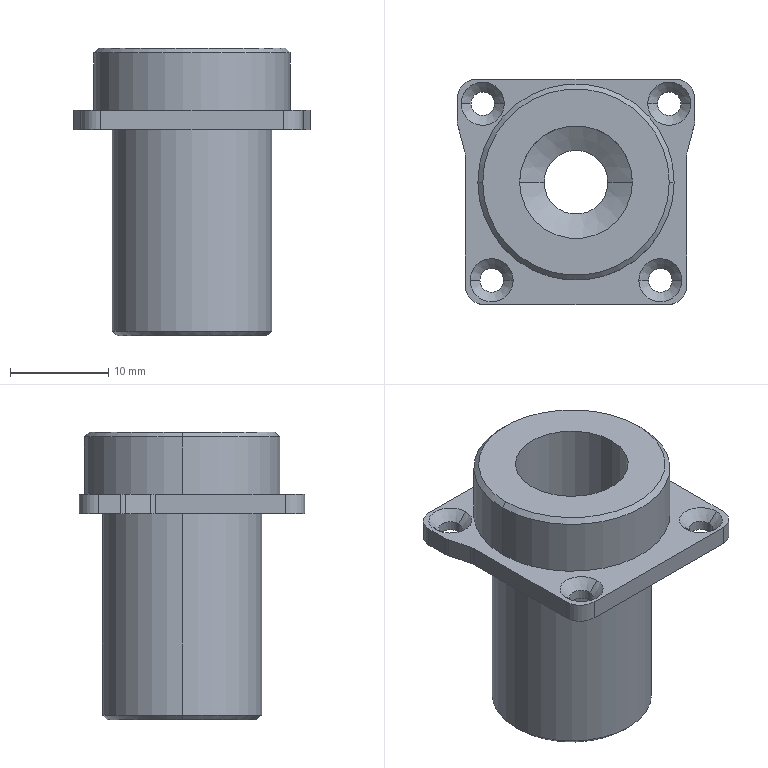NC program | NX | posted with a generic post | part box 24.2 x 23 x 29.342 mm
Lines 1 to 754 of 2259:
N10 G17 G21 G94 G90
(动态粗_2 , TOOL : D8-25-D8-60-3T-ROUGH)
N12 T02 M6
N14 G54
N16 G17 G0 G90 X-22.512 Y5.441 S6500 M3
N18 G43 Z20. H2
N20 Z-7.845
N22 G94 G1 X-22.487 Y5.442 Z-8.001 F3000.
N24 X-22.462 Y5.443 Z-8.063
N26 X-22.437 Y5.444 Z-8.109
N28 X-22.412 Y5.445 Z-8.145
N30 X-22.387 Y5.446 Z-8.176
N32 X-22.362 Y5.447 Z-8.202
N34 X-22.337 Y5.448 Z-8.225
N36 X-22.312 Y5.45 Z-8.245
N38 X-22.287 Y5.451 Z-8.263
N40 X-22.262 Y5.452 Z-8.278
N42 X-22.237 Y5.453 Z-8.292
N44 X-22.212 Y5.454 Z-8.303
N46 X-22.187 Y5.455 Z-8.314
N48 X-22.162 Y5.456 Z-8.322
N50 X-22.137 Y5.457 Z-8.329
N52 X-22.112 Y5.459 Z-8.335
N54 X-22.087 Y5.46 Z-8.34
N56 X-22.062 Y5.461 Z-8.343
N58 X-22.037 Y5.462 Z-8.345
N60 X-22.012 Y5.463
N62 X-20.703 Y5.522
N64 G3 X-20. Y6.002 R0.809
N66 X-19.572 Y8.199 R7.463
N68 X-19.395 Y13.319 R106.579
N70 G2 X-17.366 Y16.534 R4.682
N72 X-13.438 Y18.014 R9.169
N74 X-8.009 Y18.368 R38.584
N76 G1 X0.271 Y18.398
N78 X14.049 Y18.397
N80 G2 X17.314 Y16.635 R4.483
N82 X18.942 Y12.823 R8.468
N84 X19.358 Y7.581 R32.221
N86 X19.398 Y-1.284 R659.911
N88 G1 X19.397 Y-15.017
N90 G2 X17.621 Y-18.322 R4.482
N92 X13.889 Y-19.928 R8.428
N94 X8.423 Y-20.361 R32.437
N96 X-0.352 Y-20.398 R663.379
N98 G1 X-14.049 Y-20.397
N100 G2 X-17.315 Y-18.63 R4.484
N102 X-18.954 Y-14.756 R8.529
N104 X-19.359 Y-9.512 R32.975
N106 X-19.379 Y3.952 R670.697
N108 G3 X-18.957 Y8.894 R317.041
N110 G2 X-18.812 Y11.634 R51.298
N112 X-15.837 Y15.936 R6.134
N114 X-11.501 Y17.394 R11.47
N116 X-5.037 Y17.773 R48.523
N118 G1 X2.882 Y17.798
N120 X12.266 Y17.782
N122 G2 X16.841 Y14.939 R5.988
N124 X18.373 Y10.596 R11.098
N126 X18.767 Y4.449 R44.394
N128 G1 X18.798 Y-3.966
N130 X18.782 Y-13.258
N132 G2 X16.002 Y-17.798 R5.972
N134 X11.573 Y-19.376 R11.04
N136 X5.426 Y-19.767 R44.614
N138 G1 X-2.989 Y-19.798
N140 X-12.258 Y-19.783
N142 G2 X-16.766 Y-17.05 R5.959
N144 X-18.36 Y-12.674 R10.881
N146 X-18.766 Y-6.483 R43.41
N148 X-18.765 Y3.057 R288.24
N150 X-18.286 Y10.04 R540.807
N152 X-14.554 Y15.361 R7.081
N154 X-9.803 Y16.81 R13.416
N156 X-2.752 Y17.176 R58.621
N158 X10.578 Y17.182 R835.39
N160 X16.232 Y13.697 R6.869
N162 X17.769 Y9.019 R12.685
N164 X18.164 Y2.646 R49.478
N166 X18.179 Y-11.629 R815.472
N168 X14.718 Y-17.217 R6.865
N170 X9.955 Y-18.778 R12.739
N172 X3.312 Y-19.169 R51.931
N174 X-10.683 Y-19.176 R655.475
N176 X-16.201 Y-15.746 R6.857
N178 X-17.754 Y-11.114 R12.528
N180 X-18.162 Y-4.787 R47.586
N182 X-18.083 Y3.94 R125.28
N184 X-17.739 Y8.81 R94.032
N186 X-13.528 Y14.722 R7.786
N188 X-8.497 Y16.2 R14.685
N190 X-1.265 Y16.573 R62.487
N192 X9.296 Y16.571 R383.455
N194 X15.664 Y12.521 R7.559
N196 X17.18 Y7.555 R14.271
N198 X17.566 Y0.776 R56.697
N200 X17.571 Y-10.288 R389.819
N202 X13.525 Y-16.66 R7.554
N204 X8.517 Y-18.185 R14.229
N206 X1.647 Y-18.568 R57.833
N208 X-9.288 Y-18.571 R390.256
N210 X-15.634 Y-14.572 R7.543
N212 X-17.153 Y-9.744 R13.906
N214 X-17.567 Y-2.696 R55.095
N216 X-17.217 Y7.463 R91.433
N218 X-14.761 Y12.546 R8.264
N220 G1 X-14.483 Y12.885
N222 G2 X-13.313 Y13.797 R9.766
N224 X-7.944 Y15.517 R15.205
N226 X-0.852 Y15.958 R55.535
N228 X7.967 Y15.969 R285.236
N230 X13.459 Y13.7 R8.163
N232 X14.491 Y12.877 R12.481
N234 G1 X15.259 Y11.938
N236 X15.83 Y10.867
N238 G2 X16.465 Y7.974 R13.069
N240 X16.957 Y0.03 R64.584
N242 X16.966 Y-9.015 R263.202
N244 X12.547 Y-16.03 R8.091
N246 X7.395 Y-17.566 R15.148
N248 X0.12 Y-17.966 R60.98
N250 X-8.114 Y-17.961 R206.184
N252 X-15.037 Y-13.536 R8.082
N254 X-16.55 Y-8.516 R15.03
N256 X-16.96 Y-0.973 R58.274
N258 X-16.652 Y6.443 R70.854
N260 X-16.3 Y8.206 R24.664
N262 X-16.18 Y9.711 R13.074
N264 G1 X-15.827 Y10.874
N266 X-15.254 Y11.946
N268 X-14.483 Y12.885
N270 X-13.543 Y13.656
N272 X-12.471 Y14.228
N274 X-11.308 Y14.581
N276 G2 X-4.847 Y15.189 R185.641
N278 X7.07 Y15.342 R157.749
N280 X10.118 Y14.7 R10.992
N282 G1 X11.326 Y14.577
N284 X12.486 Y14.222
N286 X13.477 Y13.69
N288 X12.486 Y14.222
N290 X11.326 Y14.577
N292 G3 X6.199 Y14.972 R82.367
N294 X-7.446 Y15.01 R819.421
N296 G2 X-8.114 Y15.371 R0.802
N298 G1 X-9.01 Y16.671 Z-8.245
N300 X-9.193 Y16.933 F15000.
N302 X-9.363 Y17.204
N304 G2 X-9.18 Y18.131 R0.807
N306 X-8.379 Y16.814 R-0.8
N308 G1 X-8.857 Y16.68
N310 X-10.376 Y16.251 Z-8.345 F3000.
N312 G3 X-10.099 Y14.7 R0.8
N314 G1 X10.061
N316 X11.326 Y14.577
N318 X12.486 Y14.222
N320 X13.555 Y13.648
N322 X14.491 Y12.877
N324 X15.259 Y11.938
N326 X15.83 Y10.867
N328 X16.181 Y9.706
N330 X16.3 Y8.499
N332 G3 X16.367 Y-1.226 R300.802
N334 G2 X16.368 Y-7.896 R177.779
N336 X15.332 Y-11.87 R9.377
N338 G1 X15.027 Y-12.874
N340 X14.454 Y-13.946
N342 X13.683 Y-14.885
N344 X12.743 Y-15.656
N346 X11.671 Y-16.228
N348 X10.508 Y-16.581
N350 G3 X6.375 Y-17.049 R499.901
N352 G2 X-3.864 Y-17.379 R115.219
N354 X-7.735 Y-17.282 R36.54
N356 X-10.338 Y-16.601 R10.078
N358 X-11.674 Y-16.227 R8.73
N360 G1 X-12.746 Y-15.654
N362 X-13.685 Y-14.883
N364 X-14.456 Y-13.943
N366 X-15.028 Y-12.871
N368 G2 X-15.673 Y-10.053 R14.491
N370 X-16.333 Y-0.447 R58.318
N372 X-16.152 Y4.948 R96.408
N374 X-16.3 Y6.249 R6.163
N376 G1 Y8.229
N378 G3 X-16.247 Y5.441 R30.966
N380 G2 X-15.973 Y2.291 R13.081
N382 G3 X-15.702 Y-6.763 R98.047
N384 G1 X-15.504 Y-8.552
N386 X-15.5 Y-10.499
N388 X-15.381 Y-11.708
N390 X-15.5 Y-10.499
N392 X-15.534 Y2.547
N394 X-16.098 Y4.689
N396 G3 X-17.144 Y5.289 R0.8
N398 X-17.654 Y4.757 Z-8.297 R0.837
N400 G1 X-17.952 Y3.999 Z-8.245
N402 X-18.275 Y3.189 F15000.
N404 X-18.585 Y2.375
N406 X-18.609 Y2.177
N408 Y-3.989
N410 G3 X-17.885 Y-11.32 R37.463
N412 G1 X-17.731 Y-12.099
N414 X-17.563 Y-12.875
N416 G3 X-15.309 Y-16.66 R7.761
N418 G1 X-13.459 Y-18.369
N420 G3 X-12.311 Y-18.305 R0.8
N422 G1 X-12.182 Y-18.156
N424 X-11.149 Y-16.962 Z-8.345 F3000.
N426 G2 X-10.51 Y-16.591 R0.883
N428 G1 X-7.5 Y-16.9
N430 G3 X5.99 Y-16.7 R112.077
N432 G1 X9.299
N434 X-9.301
N436 X-9.928 Y-16.638
N438 G3 X-10.397 Y-18.132 R0.8
N440 G1 X-10.016 Y-18.283 Z-8.319
N442 X-9.629 Y-18.416 Z-8.293
N444 X-8.913 Y-18.669 Z-8.245
N446 X-7.683 Y-19.104 F15000.
N448 X-7.551 Y-19.137
N450 X-7.416 Y-19.15
N452 X8.372
N454 G3 X12.628 Y-18.396 R12.335
N456 X15.501 Y-16.541 R8.304
N458 G1 X17.108 Y-14.947
N460 G3 X17.007 Y-13.725 R0.8
N462 G1 X16.874 Y-13.632
N464 X15.587 Y-12.718 Z-8.345 F3000.
N466 G2 X15.332 Y-11.87 R0.801
N468 G3 X15.999 Y-5.757 R26.509
N470 X15.938 Y4.056 R319.266
N472 X16.285 Y6.022 R7.695
N474 G2 X15.948 Y4.118 R7.088
N476 G3 X15.5 Y0.932 R11.588
N478 G1 Y-10.501
N480 X15.38 Y-11.711
N482 X15.5 Y-10.501
N484 G2 X15.516 Y2.489 R970.595
N486 G1 X15.745 Y3.362
N488 G2 X16.658 Y3.95 R0.808
N490 G1 X17.894 Y3.745
N492 X17.919 Y3.741
N494 X17.943 Y3.737 Z-8.343
N496 X17.968 Y3.733 Z-8.34
N498 X17.993 Y3.729 Z-8.335
N500 X18.017 Y3.725 Z-8.329
N502 X18.042 Y3.721 Z-8.322
N504 X18.067 Y3.717 Z-8.314
N506 X18.091 Y3.713 Z-8.303
N508 X18.116 Y3.708 Z-8.292
N510 X18.141 Y3.704 Z-8.278
N512 X18.165 Y3.7 Z-8.263
N514 X18.19 Y3.696 Z-8.245
N516 X18.215 Y3.692 Z-8.225
N518 X18.239 Y3.688 Z-8.202
N520 X18.264 Y3.684 Z-8.176
N522 X18.289 Y3.68 Z-8.145
N524 X18.313 Y3.676 Z-8.109
N526 X18.338 Y3.672 Z-8.063
N528 X18.363 Y3.668 Z-8.001
N530 X18.387 Y3.664 Z-7.845
N532 G0 Z20.
N534 X-18.056 Y-0.544
N536 Z-5.692
N538 G1 X-18.031 Y-0.543 Z-5.848
N540 X-18.006 Y-0.541 Z-5.91
N542 X-17.981 Y-0.54 Z-5.955
N544 X-17.956 Y-0.539 Z-5.992
N546 X-17.931 Y-0.538 Z-6.023
N548 X-17.906 Y-0.537 Z-6.049
N550 X-17.881 Y-0.535 Z-6.072
N552 X-17.856 Y-0.534 Z-6.092
N554 X-17.831 Y-0.533 Z-6.11
N556 X-17.806 Y-0.532 Z-6.125
N558 X-17.781 Y-0.53 Z-6.139
N560 X-17.757 Y-0.529 Z-6.15
N562 X-17.732 Y-0.528 Z-6.16
N564 X-17.707 Y-0.527 Z-6.169
N566 X-17.682 Y-0.526 Z-6.176
N568 X-17.657 Y-0.524 Z-6.182
N570 X-17.632 Y-0.523 Z-6.186
N572 X-17.607 Y-0.522 Z-6.189
N574 X-17.582 Y-0.521 Z-6.191
N576 X-17.557 Y-0.52 Z-6.192
N578 X-16.242 Y-0.456
N580 G3 X-15.544 Y0.02 R0.809
N582 X-15.265 Y2.979 R5.282
N584 G2 X-15.573 Y7.824 R21.945
N586 X-11.556 Y13.104 R6.034
N588 X-7.333 Y13.936 R14.619
N590 X-1.626 Y14.093 R100.555
N592 X1.604 Y14.151 R18.527
N594 G1 X8.859 Y14.082
N596 G2 X13.059 Y12.48 R6.527
N598 X15.067 Y8.869 R7.229
N600 X15.196 Y4.756 R10.856
N602 G3 X14.924 Y-0.404 R42.779
N604 G2 X14.876 Y-9.366 R674.909
N606 X13.175 Y-13.57 R6.436
N608 X9.53 Y-15.501 R7.476
N610 X4.482 Y-16.039 R24.687
N612 X-8.127 Y-16.077 R423.69
N614 X-12.348 Y-14.396 R6.459
N616 X-14.299 Y-10.757 R7.365
N618 X-14.836 Y-5.8 R24.291
N620 X-14.827 Y-1.258 R45.147
N622 G3 X-14.744 Y2.734 R19.949
N624 G2 X-14.905 Y6.411 R31.666
N626 X-11.612 Y11.716 R6.376
N628 X-7.086 Y13.138 R12.123
N630 G1 X-4.76 Y13.378
N632 X-3.102 Y13.857
N634 X-1.383 Y14.132
N636 X0.403 Y14.192
N638 X2.093 Y14.045
N640 G3 X6.185 Y13.573 R18.076
N642 G2 X9.306 Y13.257 R14.034
N644 X13.888 Y8.721 R6.619
N646 X14.379 Y4.942 R12.987
N648 G1 X14.313 Y-2.676
N650 G2 X14.26 Y-8.243 R144.693
N652 X10.572 Y-13.892 R6.619
N654 X5.915 Y-15.194 R13.228
N656 X-1.185 Y-15.485 R68.155
N658 X-7.079 Y-15.455 R116.893
N660 X-12.675 Y-11.812 R6.599
N662 X-13.985 Y-7.205 R13.045
N664 X-14.149 Y-0.973 R35.635
N666 X-14.163 Y1.031 R16.707
N668 X-14.256 Y4.941 R219.386
N670 X-10.671 Y10.939 R7.006
N672 X-7.102 Y12.277 R12.297
N674 G1 X-6.377 Y12.687
N676 X-4.732 Y13.385
N678 X-6.377 Y12.687
N680 G2 X-8.857 Y11.422 R20.302
N682 G3 X-12.298 Y8.661 R8.483
N684 X-13.649 Y4.605 R8.528
N686 G2 X-13.773 Y3.456 R6.931
N688 G1 X-14.092 Y1.744
N690 X-14.167 Y0.531
N692 X-14.092 Y1.744
N694 X-13.742 Y3.554
N696 G2 X-12.416 Y6.912 R16.172
N698 X-10.517 Y9.542 R17.949
N700 G1 X-9.269 Y10.757
N702 X-7.882 Y11.811
N704 X-7.221 Y12.196
N706 X-7.882 Y11.811
N708 X-9.269 Y10.757
N710 X-10.517 Y9.542
N712 X-11.606 Y8.182
N714 X-12.52 Y6.7
N716 X-13.246 Y5.116
N718 X-13.773 Y3.456
N720 X-14.092 Y1.744
N722 X-14.2 Y0.004
N724 G3 X-13.974 Y-2.692 R28.349
N726 X-13.515 Y-7.605 R57.009
N728 X-12.028 Y-11.772 R10.612
N730 X-7.667 Y-14.66 R6.957
N732 X-3.062 Y-15.096 R22.248
N734 X5.121 Y-14.877 R76.871
N736 X9.681 Y-13.731 R13.656
N738 X13.423 Y-9.021 R6.858
N740 X13.904 Y-4.555 R20.928
N742 G1 X13.948 Y-2.531
N744 X14.103 Y-1.654
N746 X14.2 Y0.004
N748 G2 X13.998 Y5.092 R101.103
N750 G3 X13.131 Y9.065 R10.136
N752 X8.801 Y12.596 R6.693
N754 X5.116 Y13.223 R23.127
N756 X3.14 Y13.819 R10.596
N758 G2 X5.078 Y13.234 R10.018
N760 G3 X8.199 Y12.127 R272.114
N762 G2 X12.61 Y7.306 R7.44
N764 X13.059 Y5.548 R30.574
N766 X13.727 Y3.635 R21.709
N768 X14.093 Y1.655 R23.357
N770 G3 X13.727 Y3.635 R23.357
N772 X13.059 Y5.548 R21.709
N774 X11.888 Y8.013 R55.543
N776 X8.824 Y11.12 R8.285
N778 G1 X7.251 Y12.209
N780 X5.616 Y13.042
N782 X7.251 Y12.209
N784 X8.824 Y11.12
N786 X10.133 Y9.948
N788 X11.331 Y8.558
N790 X12.34 Y7.025
N792 X13.143 Y5.375
N794 X13.727 Y3.635
N796 X14.081 Y1.835
N798 X14.2 Y0.004
N800 G2 X13.814 Y-3.29 R16.567
N802 G3 X13.323 Y-5.938 R16.464
N804 G2 X12.42 Y-9.408 R11.858
N806 X8.318 Y-13.166 R7.767
N808 X3.42 Y-14.277 R16.444
N810 X-5.209 Y-14.332 R51.279
N812 X-9.147 Y-13.043 R8.477
N814 X-12.198 Y-8.926 R8.259
N816 X-12.984 Y-5.74 R18.647
N818 X-14.055 Y-1.907 R14.192
N820 G3 X-12.804 Y-6.147 R14.594
N822 X-11.609 Y-9.212 R35.123
N824 X-6.191 Y-13.549 R7.933
N826 X-1.88 Y-14.058 R19.593
N828 G1 X-0.404 Y-14.194
N830 G3 X6.165 Y-13.399 R29.845
N832 X10.388 Y-11.103 R9.034
N834 X12.558 Y-7.054 R9.04
N836 G1 X12.801 Y-6.112
N838 G3 X13.711 Y-3.63 R13.2
N840 G2 X12.801 Y-6.112 R13.081
N842 X11.84 Y-7.839 R16.008
N844 X8.28 Y-11.519 R9.586
N846 G1 X8.083 Y-11.675
N848 X6.542 Y-12.603
N850 X4.895 Y-13.329
N852 X3.17 Y-13.841
N854 X1.395 Y-14.131
N856 X3.17 Y-13.841
N858 X4.895 Y-13.329
N860 X6.542 Y-12.603
N862 X8.083 Y-11.675
N864 X9.494 Y-10.559
N866 X10.753 Y-9.274
N868 X11.84 Y-7.839
N870 G2 X13.069 Y-7.784 R0.8
N872 X13.268 Y-8.467 Z-6.145 R0.84
N874 G1 X13.196 Y-9.307 Z-6.092
N876 X13.076 Y-10.699 F15000.
N878 G2 X12.759 Y-11.271 R0.803
N880 G1 X11.494 Y-12.224
N882 X10.218 Y-13.163
N884 G2 X6.565 Y-15.249 R22.592
N886 X4.719 Y-15.989 R14.369
N888 X2.475 Y-16.419 R10.72
N890 G1 X0.632 Y-16.57
N892 G2 X-0.125 Y-16.177 R0.805
N894 G1 X-0.993 Y-14.858 Z-6.192 F3000.
N896 X-1.169 Y-14.585
N898 X-1.358 Y-14.32
N900 G3 X-1.88 Y-14.058 R0.805
N902 G1 X-2.195 Y-14.029
N904 G2 X-6.949 Y-12.534 R20.191
N906 X-9.68 Y-10.357 R8.581
N908 G1 X-10.079 Y-10.003
N910 X-11.263 Y-8.648
N912 X-12.266 Y-7.154
N914 X-12.925 Y-5.874
N916 X-12.266 Y-7.154
N918 X-11.263 Y-8.648
N920 X-10.079 Y-10.003
N922 X-8.733 Y-11.197
N924 X-7.247 Y-12.211
N926 X-5.645 Y-13.03
N928 X-4.205 Y-13.548
N930 G2 X-3.673 Y-14.371 R0.808
N932 G1 X-3.777 Y-15.699
N934 X-3.779 Y-15.724 Z-6.191
N936 X-3.781 Y-15.749 Z-6.189
N938 X-3.783 Y-15.774 Z-6.186
N940 X-3.785 Y-15.799 Z-6.182
N942 X-3.787 Y-15.824 Z-6.176
N944 X-3.789 Y-15.849 Z-6.169
N946 X-3.791 Y-15.874 Z-6.16
N948 X-3.793 Y-15.899 Z-6.15
N950 X-3.795 Y-15.924 Z-6.139
N952 X-3.797 Y-15.949 Z-6.125
N954 X-3.799 Y-15.974 Z-6.11
N956 X-3.8 Y-15.998 Z-6.092
N958 X-3.802 Y-16.023 Z-6.072
N960 X-3.804 Y-16.048 Z-6.049
N962 X-3.806 Y-16.073 Z-6.023
N964 X-3.808 Y-16.098 Z-5.992
N966 X-3.81 Y-16.123 Z-5.955
N968 X-3.812 Y-16.148 Z-5.91
N970 X-3.814 Y-16.173 Z-5.848
N972 X-3.816 Y-16.198 Z-5.692
N974 G0 Z20.
N976 X-16.722 Y-0.554
N978 Z0.407
N980 G1 X-16.697 Z0.251
N982 X-16.672 Z0.189
N984 X-16.647 Y-0.553 Z0.144
N986 X-16.622 Z0.107
N988 X-16.597 Z0.076
N990 X-16.572 Y-0.552 Z0.05
N992 X-16.547 Z0.027
N994 X-16.522 Z0.007
N996 X-16.497 Z-0.01
N998 X-16.472 Y-0.551 Z-0.026
N1000 X-16.447 Z-0.039
N1002 X-16.422 Z-0.051
N1004 X-16.397 Y-0.55 Z-0.061
N1006 X-16.372 Z-0.07
N1008 X-16.347 Z-0.077
N1010 X-16.322 Y-0.549 Z-0.083
N1012 X-16.297 Z-0.087
N1014 X-16.272 Z-0.09
N1016 X-16.247 Y-0.548 Z-0.092
N1018 X-16.222 Z-0.093
N1020 X-14.956 Y-0.533
N1022 G3 X-14.209 Y-0.009 R0.809
N1024 X-13.769 Y1.327 R32.004
N1026 G1 X-13.74 Y1.78
N1028 X-13.399 Y3.525
N1030 X-12.837 Y5.212
N1032 X-12.064 Y6.813
N1034 X-11.092 Y8.302
N1036 X-9.937 Y9.654
N1038 X-8.619 Y10.848
N1040 X-7.159 Y11.862
N1042 X-5.581 Y12.681
N1044 X-3.91 Y13.292
N1046 X-2.176 Y13.683
N1048 X-0.405 Y13.849
N1050 X1.372 Y13.787
N1052 X3.126 Y13.498
N1054 X4.746 Y13.016
N1056 X6.296 Y12.342
N1058 X7.753 Y11.483
N1060 X9.093 Y10.453
N1062 X10.299 Y9.268
N1064 X11.351 Y7.945
N1066 X12.234 Y6.503
N1068 X12.935 Y4.965
N1070 X13.443 Y3.353
N1072 X13.751 Y1.691
N1074 X13.855 Y0.004
N1076 G2 X13.461 Y-3.281 R16.145
N1078 X12.3 Y-6.378 R16.145
N1080 G1 X11.45 Y-7.801
N1082 X10.388 Y-9.168
N1084 X9.163 Y-10.392
N1086 X7.795 Y-11.454
N1088 X6.306 Y-12.337
N1090 X4.718 Y-13.027
N1092 X3.056 Y-13.514
N1094 X1.346 Y-13.789
N1096 X-0.384 Y-13.85
N1098 X-2.109 Y-13.693
N1100 X-3.8 Y-13.323
N1102 X-5.433 Y-12.745
N1104 X-6.98 Y-11.968
N1106 X-8.418 Y-11.004
N1108 X-9.725 Y-9.868
N1110 X-10.88 Y-8.578
N1112 X-11.865 Y-7.154
N1114 G2 X-13.774 Y-1.496 R14.451
N1116 X-13.768 Y1.352 R14.237
N1118 G3 X-14.322 Y2.171 R0.808
N1120 G1 X-15.593 Y2.589
N1122 X-15.616 Y2.597 Z-0.092
N1124 X-15.64 Y2.605 Z-0.09
N1126 X-15.664 Y2.612 Z-0.087
N1128 X-15.688 Y2.62 Z-0.083
N1130 X-15.712 Y2.628 Z-0.077
N1132 X-15.735 Y2.636 Z-0.07
N1134 X-15.759 Y2.644 Z-0.061
N1136 X-15.783 Y2.651 Z-0.051
N1138 X-15.807 Y2.659 Z-0.039
N1140 X-15.83 Y2.667 Z-0.026
N1142 X-15.854 Y2.675 Z-0.01
N1144 X-15.878 Y2.683 Z0.007
N1146 X-15.902 Y2.69 Z0.027
N1148 X-15.925 Y2.698 Z0.05
N1150 X-15.949 Y2.706 Z0.076
N1152 X-15.973 Y2.714 Z0.107
N1154 X-15.997 Y2.722 Z0.144
N1156 X-16.02 Y2.729 Z0.189
N1158 X-16.044 Y2.737 Z0.251
N1160 X-16.068 Y2.745 Z0.407
N1162 G0 Z20.
N1164 X-16.37 Y-1.525
N1166 Z0.65
N1168 G1 X-16.345 Y-1.526 Z0.494
N1170 X-16.32 Y-1.527 Z0.432
N1172 X-16.295 Y-1.528 Z0.387
N1174 X-16.27 Y-1.529 Z0.35
N1176 X-16.245 Y-1.53 Z0.319
N1178 X-16.22 Y-1.531 Z0.293
N1180 X-16.195 Y-1.532 Z0.27
N1182 X-16.17 Y-1.533 Z0.25
N1184 X-16.145 Y-1.534 Z0.232
N1186 X-16.12 Y-1.535 Z0.217
N1188 X-16.095 Y-1.536 Z0.203
N1190 X-16.07 Y-1.537 Z0.192
N1192 X-16.045 Y-1.538 Z0.182
N1194 X-16.02 Y-1.539 Z0.173
N1196 X-15.995 Y-1.54 Z0.166
N1198 X-15.97 Y-1.541 Z0.16
N1200 X-15.945 Y-1.542 Z0.156
N1202 X-15.92 Y-1.543 Z0.153
N1204 X-15.896 Y-1.544 Z0.151
N1206 X-15.871 Y-1.545 Z0.15
N1208 X-14.632 Y-1.594
N1210 G3 X-13.819 Y-0.995 R0.808
N1212 X-13.056 Y2.174 R56.521
N1214 G2 X-9.146 Y9.274 R14.704
N1216 X-12.357 Y-4.078 R-13.014
N1218 X-12.575 Y0.473 R10.987
N1220 X-8.371 Y8.876 R13.895
N1222 X5.39 Y-10.912 R-12.182
N1224 X-10.945 Y-5.283 R12.121
N1226 X-11.573 Y1.381 R11.239
N1228 X-4.72 Y10.29 R12.195
N1230 X-8.878 Y-6.985 R-11.303
N1232 X-10.783 Y0.813 R10.286
N1234 X-3.054 Y9.967 R11.138
N1236 X-6.826 Y-7.84 R-10.404
N1238 X-9.821 Y1.045 R9.593
N1240 X-0.833 Y9.443 R10.042
N1242 X-5.164 Y-7.904 R-9.458
N1244 X-8.687 Y1.727 R8.815
N1246 X1.218 Y8.387 R8.927
N1248 X-3.127 Y-7.827 R-8.451
N1250 X-7.206 Y2.793 R7.891
N1252 X3.015 Y6.726 R7.736
N1254 X-1.082 Y-7.229 R7.341
N1256 X-1.782 Y5.977 R6.766
N1258 X5.827 Y-1.536 R6.185
N1260 X-1.144 Y-5.804 R5.862
N1262 X-3.913 Y2.96 R5.346
N1264 X2.857 Y3.245 R4.707
N1266 X3.198 Y-2.39 R4.138
N1268 X-0.278 Y-3.389 R3.352
N1270 G1 X-0.497 Y-3.338
N1272 X-0.522 Y-3.332 Z0.151
N1274 X-0.546 Y-3.327 Z0.153
N1276 X-0.57 Y-3.321 Z0.156
N1278 X-0.595 Y-3.315 Z0.16
N1280 X-0.619 Y-3.31 Z0.166
N1282 X-0.644 Y-3.304 Z0.173
N1284 X-0.668 Y-3.299 Z0.182
N1286 X-0.692 Y-3.293 Z0.192
N1288 X-0.717 Y-3.288 Z0.203
N1290 X-0.741 Y-3.282 Z0.217
N1292 X-0.765 Y-3.276 Z0.232
N1294 X-0.79 Y-3.271 Z0.25
N1296 X-0.814 Y-3.265 Z0.27
N1298 X-0.839 Y-3.26 Z0.293
N1300 X-0.863 Y-3.254 Z0.319
N1302 X-0.887 Y-3.249 Z0.35
N1304 X-0.912 Y-3.243 Z0.387
N1306 X-0.936 Y-3.238 Z0.432
N1308 X-0.96 Y-3.232 Z0.494
N1310 X-0.985 Y-3.226 Z0.65
N1312 G0 Z20.
N1314 M5
(PLANAR_MILL_3_COPY , TOOL : D8-25-D8-60-3T-FINISH)
N1316 T03 M6
N1318 G54
N1320 G17 G0 G90 X-13.604 Y-2. S5500 M3
N1322 G43 Z20. H3
N1324 Z2.05
N1326 G94 G1 Z0.05 F800.
N1328 X-10.75
N1330 G3 X-8.75 Y0. R2.
N1332 G2 X0. Y8.75 R8.75
N1334 X-8.75 Y0. R-8.75
N1336 G3 X-10.75 Y2. R2.
N1338 G1 X-13.604
N1340 Z2.05
N1342 G0 Z20.
(PLANAR_MILL_3_COPY_COPY , TOOL : D8-25-D8-60-3T-FINISH)
N1344 Y-2.
N1346 Z2.
N1348 G1 Z0.
N1350 X-10.75
N1352 G3 X-8.75 Y0. R2.
N1354 G2 X0. Y8.75 R8.75
N1356 X-8.75 Y0. R-8.75
N1358 G3 X-10.75 Y2. R2.
N1360 G1 X-13.604
N1362 Z2.
N1364 G0 Z20.
(PLANAR_MILL_3 , TOOL : D8-25-D8-60-3T-FINISH)
N1366 X16. S5000
N1368 Z-4.342
N1370 G1 Z-6.342 F500.
N1372 G3 X14. Y0. R2.
N1374 G2 X0. Y-14. R14.
N1376 X14. Y0. R-14.
N1378 G3 X16. Y-2. R2.
N1380 G1 Y2.
N1382 G3 X14. Y0. R2.
N1384 G2 X0. Y-14. R14.
N1386 X14. Y0. R-14.
N1388 G3 X16. Y-2. R2.
N1390 G1 Z-4.342
N1392 G0 Z20.
(PLANAR_MILL_2 , TOOL : D8-25-D8-60-3T-FINISH)
N1394 X10.265 Y-17.697 S5500
N1396 Z-6.442
N1398 G1 Z-8.442
N1400 G41 X10.3 Y-17.5 D3
N1402 G3 X9.3 Y-16.5 R1.
N1404 G1 X-9.3
N1406 G2 X-15.3 Y-10.5 R6.
N1408 G1 Y2.473
N1410 X-15.896 Y4.696
N1412 G2 X-16.1 Y6.249 R6.
N1414 G1 Y8.5
N1416 G2 X-10.1 Y14.5 R6.
N1418 G1 X10.1
N1420 G2 X16.1 Y8.5 R6.
N1422 G1 Y6.249
N1424 G2 X15.896 Y4.696 R6.
N1426 G1 X15.3 Y2.473
N1428 Y-10.5
N1430 G2 X9.3 Y-16.5 R6.
N1432 G3 X8.3 Y-17.5 R1.
N1434 G40
N1436 G1 X8.335 Y-17.697
N1438 X10.265
N1440 G41 X10.3 Y-17.5
N1442 G3 X9.3 Y-16.5 R1.
N1444 G1 X-9.3
N1446 G2 X-15.3 Y-10.5 R6.
N1448 G1 Y2.473
N1450 X-15.896 Y4.696
N1452 G2 X-16.1 Y6.249 R6.
N1454 G1 Y8.5
N1456 G2 X-10.1 Y14.5 R6.
N1458 G1 X10.1
N1460 G2 X16.1 Y8.5 R6.
N1462 G1 Y6.249
N1464 G2 X15.896 Y4.696 R6.
N1466 G1 X15.3 Y2.473
N1468 Y-10.5
N1470 G2 X9.3 Y-16.5 R6.
N1472 G3 X8.3 Y-17.5 R1.
N1474 G40
N1476 G1 X8.335 Y-17.697
N1478 Z-6.442
N1480 G0 Z20.
N1482 M5